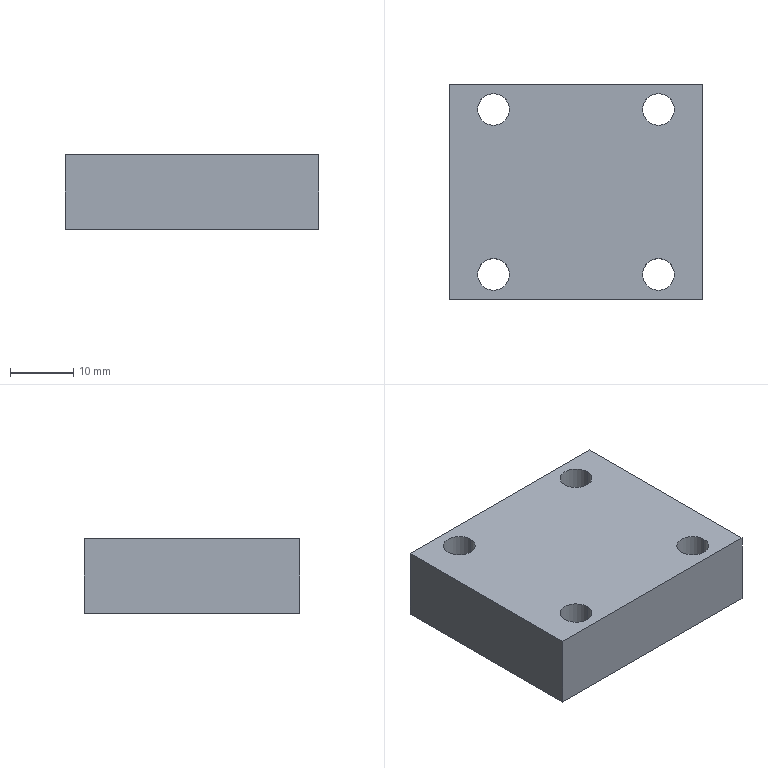Part | NX | 1 solid | 14 faces | box 40 x 34 x 11.7 mm | volume 14993 mm3 | cylinder 8 | plane 6 | commonest cylinder face diameters 5 x8
STEP:
#1=CARTESIAN_POINT('',(0.,-34.,12.3));
#2=VERTEX_POINT('',#1);
#3=CARTESIAN_POINT('',(0.,0.,12.3));
#4=VERTEX_POINT('',#3);
#5=CARTESIAN_POINT('',(0.,0.,12.3));
#6=DIRECTION('',(0.,1.,0.));
#7=VECTOR('',#6,1000.);
#8=LINE('',#5,#7);
#9=EDGE_CURVE('',#2,#4,#8,.T.);
#10=ORIENTED_EDGE('',*,*,#9,.F.);
#11=CARTESIAN_POINT('',(40.,-34.,12.3));
#12=VERTEX_POINT('',#11);
#13=CARTESIAN_POINT('',(0.,-34.,12.3));
#14=DIRECTION('',(1.,0.,0.));
#15=VECTOR('',#14,1000.);
#16=LINE('',#13,#15);
#17=EDGE_CURVE('',#2,#12,#16,.T.);
#18=ORIENTED_EDGE('',*,*,#17,.T.);
#19=CARTESIAN_POINT('',(40.,0.,12.3));
#20=VERTEX_POINT('',#19);
#21=CARTESIAN_POINT('',(40.,0.,12.3));
#22=DIRECTION('',(0.,-1.,0.));
#23=VECTOR('',#22,1000.);
#24=LINE('',#21,#23);
#25=EDGE_CURVE('',#20,#12,#24,.T.);
#26=ORIENTED_EDGE('',*,*,#25,.F.);
#27=CARTESIAN_POINT('',(0.,0.,12.3));
#28=DIRECTION('',(1.,0.,0.));
#29=VECTOR('',#28,1000.);
#30=LINE('',#27,#29);
#31=EDGE_CURVE('',#4,#20,#30,.T.);
#32=ORIENTED_EDGE('',*,*,#31,.F.);
#33=EDGE_LOOP('',(#10,#18,#26,#32));
#34=FACE_BOUND('',#33,.T.);
#35=CARTESIAN_POINT('',(4.5,-4.,12.3));
#36=VERTEX_POINT('',#35);
#37=CARTESIAN_POINT('',(9.5,-4.,12.3));
#38=VERTEX_POINT('',#37);
#39=CARTESIAN_POINT('',(7.,-4.,12.3));
#40=DIRECTION('',(0.,0.,-1.));
#41=DIRECTION('',(-1.,0.,0.));
#42=AXIS2_PLACEMENT_3D('',#39,#40,#41);
#43=CIRCLE('',#42,2.5);
#44=EDGE_CURVE('',#36,#38,#43,.T.);
#45=ORIENTED_EDGE('',*,*,#44,.T.);
#46=CARTESIAN_POINT('',(7.,-4.,12.3));
#47=DIRECTION('',(0.,0.,-1.));
#48=DIRECTION('',(-1.,0.,0.));
#49=AXIS2_PLACEMENT_3D('',#46,#47,#48);
#50=CIRCLE('',#49,2.5);
#51=EDGE_CURVE('',#38,#36,#50,.T.);
#52=ORIENTED_EDGE('',*,*,#51,.T.);
#53=EDGE_LOOP('',(#45,#52));
#54=FACE_BOUND('',#53,.T.);
#55=CARTESIAN_POINT('',(35.5,-30.,12.3));
#56=VERTEX_POINT('',#55);
#57=CARTESIAN_POINT('',(30.5,-30.,12.3));
#58=VERTEX_POINT('',#57);
#59=CARTESIAN_POINT('',(33.,-30.,12.3));
#60=DIRECTION('',(0.,0.,-1.));
#61=DIRECTION('',(-1.,0.,0.));
#62=AXIS2_PLACEMENT_3D('',#59,#60,#61);
#63=CIRCLE('',#62,2.5);
#64=EDGE_CURVE('',#56,#58,#63,.T.);
#65=ORIENTED_EDGE('',*,*,#64,.T.);
#66=CARTESIAN_POINT('',(33.,-30.,12.3));
#67=DIRECTION('',(0.,0.,-1.));
#68=DIRECTION('',(-1.,0.,0.));
#69=AXIS2_PLACEMENT_3D('',#66,#67,#68);
#70=CIRCLE('',#69,2.5);
#71=EDGE_CURVE('',#58,#56,#70,.T.);
#72=ORIENTED_EDGE('',*,*,#71,.T.);
#73=EDGE_LOOP('',(#65,#72));
#74=FACE_BOUND('',#73,.T.);
#75=CARTESIAN_POINT('',(35.5,-4.,12.3));
#76=VERTEX_POINT('',#75);
#77=CARTESIAN_POINT('',(30.5,-4.,12.3));
#78=VERTEX_POINT('',#77);
#79=CARTESIAN_POINT('',(33.,-4.,12.3));
#80=DIRECTION('',(0.,0.,-1.));
#81=DIRECTION('',(-1.,0.,0.));
#82=AXIS2_PLACEMENT_3D('',#79,#80,#81);
#83=CIRCLE('',#82,2.5);
#84=EDGE_CURVE('',#76,#78,#83,.T.);
#85=ORIENTED_EDGE('',*,*,#84,.T.);
#86=CARTESIAN_POINT('',(33.,-4.,12.3));
#87=DIRECTION('',(0.,0.,-1.));
#88=DIRECTION('',(-1.,0.,0.));
#89=AXIS2_PLACEMENT_3D('',#86,#87,#88);
#90=CIRCLE('',#89,2.5);
#91=EDGE_CURVE('',#78,#76,#90,.T.);
#92=ORIENTED_EDGE('',*,*,#91,.T.);
#93=EDGE_LOOP('',(#85,#92));
#94=FACE_BOUND('',#93,.T.);
#95=CARTESIAN_POINT('',(9.5,-30.,12.3));
#96=VERTEX_POINT('',#95);
#97=CARTESIAN_POINT('',(4.5,-30.,12.3));
#98=VERTEX_POINT('',#97);
#99=CARTESIAN_POINT('',(7.,-30.,12.3));
#100=DIRECTION('',(0.,0.,-1.));
#101=DIRECTION('',(-1.,0.,0.));
#102=AXIS2_PLACEMENT_3D('',#99,#100,#101);
#103=CIRCLE('',#102,2.5);
#104=EDGE_CURVE('',#96,#98,#103,.T.);
#105=ORIENTED_EDGE('',*,*,#104,.T.);
#106=CARTESIAN_POINT('',(7.,-30.,12.3));
#107=DIRECTION('',(0.,0.,-1.));
#108=DIRECTION('',(-1.,0.,0.));
#109=AXIS2_PLACEMENT_3D('',#106,#107,#108);
#110=CIRCLE('',#109,2.5);
#111=EDGE_CURVE('',#98,#96,#110,.T.);
#112=ORIENTED_EDGE('',*,*,#111,.T.);
#113=EDGE_LOOP('',(#105,#112));
#114=FACE_BOUND('',#113,.T.);
#115=CARTESIAN_POINT('',(0.,0.,12.3));
#116=DIRECTION('',(0.,0.,1.));
#117=DIRECTION('',(1.,0.,0.));
#118=AXIS2_PLACEMENT_3D('',#115,#116,#117);
#119=PLANE('',#118);
#120=ADVANCED_FACE('',(#34,#54,#74,#94,#114),#119,.T.);
#121=CARTESIAN_POINT('',(0.,0.,0.6));
#122=VERTEX_POINT('',#121);
#123=CARTESIAN_POINT('',(0.,-34.,0.6));
#124=VERTEX_POINT('',#123);
#125=CARTESIAN_POINT('',(0.,0.,0.6));
#126=DIRECTION('',(0.,-1.,0.));
#127=VECTOR('',#126,1000.);
#128=LINE('',#125,#127);
#129=EDGE_CURVE('',#122,#124,#128,.T.);
#130=ORIENTED_EDGE('',*,*,#129,.T.);
#131=CARTESIAN_POINT('',(0.,-34.,0.));
#132=DIRECTION('',(0.,0.,1.));
#133=VECTOR('',#132,1000.);
#134=LINE('',#131,#133);
#135=EDGE_CURVE('',#124,#2,#134,.T.);
#136=ORIENTED_EDGE('',*,*,#135,.T.);
#137=ORIENTED_EDGE('',*,*,#9,.T.);
#138=CARTESIAN_POINT('',(0.,0.,0.));
#139=DIRECTION('',(0.,0.,1.));
#140=VECTOR('',#139,1000.);
#141=LINE('',#138,#140);
#142=EDGE_CURVE('',#122,#4,#141,.T.);
#143=ORIENTED_EDGE('',*,*,#142,.F.);
#144=EDGE_LOOP('',(#130,#136,#137,#143));
#145=FACE_BOUND('',#144,.T.);
#146=CARTESIAN_POINT('',(0.,0.,0.));
#147=DIRECTION('',(-1.,0.,0.));
#148=DIRECTION('',(0.,0.,1.));
#149=AXIS2_PLACEMENT_3D('',#146,#147,#148);
#150=PLANE('',#149);
#151=ADVANCED_FACE('',(#145),#150,.T.);
#152=CARTESIAN_POINT('',(40.,0.,0.6));
#153=VERTEX_POINT('',#152);
#154=CARTESIAN_POINT('',(0.,0.,0.6));
#155=DIRECTION('',(-1.,0.,0.));
#156=VECTOR('',#155,1000.);
#157=LINE('',#154,#156);
#158=EDGE_CURVE('',#153,#122,#157,.T.);
#159=ORIENTED_EDGE('',*,*,#158,.T.);
#160=ORIENTED_EDGE('',*,*,#142,.T.);
#161=ORIENTED_EDGE('',*,*,#31,.T.);
#162=CARTESIAN_POINT('',(40.,0.,0.));
#163=DIRECTION('',(0.,0.,-1.));
#164=VECTOR('',#163,1000.);
#165=LINE('',#162,#164);
#166=EDGE_CURVE('',#20,#153,#165,.T.);
#167=ORIENTED_EDGE('',*,*,#166,.T.);
#168=EDGE_LOOP('',(#159,#160,#161,#167));
#169=FACE_BOUND('',#168,.T.);
#170=CARTESIAN_POINT('',(40.,0.,0.));
#171=DIRECTION('',(0.,1.,0.));
#172=DIRECTION('',(1.,0.,0.));
#173=AXIS2_PLACEMENT_3D('',#170,#171,#172);
#174=PLANE('',#173);
#175=ADVANCED_FACE('',(#169),#174,.T.);
#176=CARTESIAN_POINT('',(40.,-34.,0.6));
#177=VERTEX_POINT('',#176);
#178=CARTESIAN_POINT('',(40.,0.,0.6));
#179=DIRECTION('',(0.,1.,0.));
#180=VECTOR('',#179,1000.);
#181=LINE('',#178,#180);
#182=EDGE_CURVE('',#177,#153,#181,.T.);
#183=ORIENTED_EDGE('',*,*,#182,.T.);
#184=ORIENTED_EDGE('',*,*,#166,.F.);
#185=ORIENTED_EDGE('',*,*,#25,.T.);
#186=CARTESIAN_POINT('',(40.,-34.,0.));
#187=DIRECTION('',(0.,0.,-1.));
#188=VECTOR('',#187,1000.);
#189=LINE('',#186,#188);
#190=EDGE_CURVE('',#12,#177,#189,.T.);
#191=ORIENTED_EDGE('',*,*,#190,.T.);
#192=EDGE_LOOP('',(#183,#184,#185,#191));
#193=FACE_BOUND('',#192,.T.);
#194=CARTESIAN_POINT('',(40.,-34.,0.));
#195=DIRECTION('',(1.,0.,0.));
#196=DIRECTION('',(0.,1.,0.));
#197=AXIS2_PLACEMENT_3D('',#194,#195,#196);
#198=PLANE('',#197);
#199=ADVANCED_FACE('',(#193),#198,.T.);
#200=CARTESIAN_POINT('',(0.,-34.,0.6));
#201=DIRECTION('',(1.,0.,0.));
#202=VECTOR('',#201,1000.);
#203=LINE('',#200,#202);
#204=EDGE_CURVE('',#124,#177,#203,.T.);
#205=ORIENTED_EDGE('',*,*,#204,.T.);
#206=ORIENTED_EDGE('',*,*,#190,.F.);
#207=ORIENTED_EDGE('',*,*,#17,.F.);
#208=ORIENTED_EDGE('',*,*,#135,.F.);
#209=EDGE_LOOP('',(#205,#206,#207,#208));
#210=FACE_BOUND('',#209,.T.);
#211=CARTESIAN_POINT('',(0.,-34.,0.));
#212=DIRECTION('',(0.,-1.,0.));
#213=DIRECTION('',(0.,0.,-1.));
#214=AXIS2_PLACEMENT_3D('',#211,#212,#213);
#215=PLANE('',#214);
#216=ADVANCED_FACE('',(#210),#215,.T.);
#217=ORIENTED_EDGE('',*,*,#129,.F.);
#218=ORIENTED_EDGE('',*,*,#158,.F.);
#219=ORIENTED_EDGE('',*,*,#182,.F.);
#220=ORIENTED_EDGE('',*,*,#204,.F.);
#221=EDGE_LOOP('',(#217,#218,#219,#220));
#222=FACE_BOUND('',#221,.T.);
#223=CARTESIAN_POINT('',(9.5,-4.,0.6));
#224=VERTEX_POINT('',#223);
#225=CARTESIAN_POINT('',(4.5,-4.,0.6));
#226=VERTEX_POINT('',#225);
#227=CARTESIAN_POINT('',(7.,-4.,0.6));
#228=DIRECTION('',(0.,0.,-1.));
#229=DIRECTION('',(-1.,0.,0.));
#230=AXIS2_PLACEMENT_3D('',#227,#228,#229);
#231=CIRCLE('',#230,2.5);
#232=EDGE_CURVE('',#224,#226,#231,.T.);
#233=ORIENTED_EDGE('',*,*,#232,.F.);
#234=CARTESIAN_POINT('',(7.,-4.,0.6));
#235=DIRECTION('',(0.,0.,-1.));
#236=DIRECTION('',(-1.,0.,0.));
#237=AXIS2_PLACEMENT_3D('',#234,#235,#236);
#238=CIRCLE('',#237,2.5);
#239=EDGE_CURVE('',#226,#224,#238,.T.);
#240=ORIENTED_EDGE('',*,*,#239,.F.);
#241=EDGE_LOOP('',(#233,#240));
#242=FACE_BOUND('',#241,.T.);
#243=CARTESIAN_POINT('',(30.5,-30.,0.6));
#244=VERTEX_POINT('',#243);
#245=CARTESIAN_POINT('',(35.5,-30.,0.6));
#246=VERTEX_POINT('',#245);
#247=CARTESIAN_POINT('',(33.,-30.,0.6));
#248=DIRECTION('',(0.,0.,-1.));
#249=DIRECTION('',(-1.,0.,0.));
#250=AXIS2_PLACEMENT_3D('',#247,#248,#249);
#251=CIRCLE('',#250,2.5);
#252=EDGE_CURVE('',#244,#246,#251,.T.);
#253=ORIENTED_EDGE('',*,*,#252,.F.);
#254=CARTESIAN_POINT('',(33.,-30.,0.6));
#255=DIRECTION('',(0.,0.,-1.));
#256=DIRECTION('',(-1.,0.,0.));
#257=AXIS2_PLACEMENT_3D('',#254,#255,#256);
#258=CIRCLE('',#257,2.5);
#259=EDGE_CURVE('',#246,#244,#258,.T.);
#260=ORIENTED_EDGE('',*,*,#259,.F.);
#261=EDGE_LOOP('',(#253,#260));
#262=FACE_BOUND('',#261,.T.);
#263=CARTESIAN_POINT('',(35.5,-4.,0.6));
#264=VERTEX_POINT('',#263);
#265=CARTESIAN_POINT('',(30.5,-4.,0.6));
#266=VERTEX_POINT('',#265);
#267=CARTESIAN_POINT('',(33.,-4.,0.6));
#268=DIRECTION('',(0.,0.,-1.));
#269=DIRECTION('',(-1.,0.,0.));
#270=AXIS2_PLACEMENT_3D('',#267,#268,#269);
#271=CIRCLE('',#270,2.5);
#272=EDGE_CURVE('',#264,#266,#271,.T.);
#273=ORIENTED_EDGE('',*,*,#272,.F.);
#274=CARTESIAN_POINT('',(33.,-4.,0.6));
#275=DIRECTION('',(0.,0.,-1.));
#276=DIRECTION('',(-1.,0.,0.));
#277=AXIS2_PLACEMENT_3D('',#274,#275,#276);
#278=CIRCLE('',#277,2.5);
#279=EDGE_CURVE('',#266,#264,#278,.T.);
#280=ORIENTED_EDGE('',*,*,#279,.F.);
#281=EDGE_LOOP('',(#273,#280));
#282=FACE_BOUND('',#281,.T.);
#283=CARTESIAN_POINT('',(9.5,-30.,0.6));
#284=VERTEX_POINT('',#283);
#285=CARTESIAN_POINT('',(4.5,-30.,0.6));
#286=VERTEX_POINT('',#285);
#287=CARTESIAN_POINT('',(7.,-30.,0.6));
#288=DIRECTION('',(0.,0.,-1.));
#289=DIRECTION('',(-1.,0.,0.));
#290=AXIS2_PLACEMENT_3D('',#287,#288,#289);
#291=CIRCLE('',#290,2.5);
#292=EDGE_CURVE('',#284,#286,#291,.T.);
#293=ORIENTED_EDGE('',*,*,#292,.F.);
#294=CARTESIAN_POINT('',(7.,-30.,0.6));
#295=DIRECTION('',(0.,0.,-1.));
#296=DIRECTION('',(-1.,0.,0.));
#297=AXIS2_PLACEMENT_3D('',#294,#295,#296);
#298=CIRCLE('',#297,2.5);
#299=EDGE_CURVE('',#286,#284,#298,.T.);
#300=ORIENTED_EDGE('',*,*,#299,.F.);
#301=EDGE_LOOP('',(#293,#300));
#302=FACE_BOUND('',#301,.T.);
#303=CARTESIAN_POINT('',(0.,0.,0.6));
#304=DIRECTION('',(0.,0.,1.));
#305=DIRECTION('',(1.,0.,0.));
#306=AXIS2_PLACEMENT_3D('',#303,#304,#305);
#307=PLANE('',#306);
#308=ADVANCED_FACE('',(#222,#242,#262,#282,#302),#307,.F.);
#309=ORIENTED_EDGE('',*,*,#232,.T.);
#310=CARTESIAN_POINT('',(4.5,-4.,3.7));
#311=DIRECTION('',(0.,0.,-1.));
#312=VECTOR('',#311,1000.);
#313=LINE('',#310,#312);
#314=EDGE_CURVE('',#226,#36,#313,.F.);
#315=ORIENTED_EDGE('',*,*,#314,.T.);
#316=ORIENTED_EDGE('',*,*,#51,.F.);
#317=CARTESIAN_POINT('',(9.5,-4.,3.7));
#318=DIRECTION('',(0.,0.,-1.));
#319=VECTOR('',#318,1000.);
#320=LINE('',#317,#319);
#321=EDGE_CURVE('',#224,#38,#320,.F.);
#322=ORIENTED_EDGE('',*,*,#321,.F.);
#323=EDGE_LOOP('',(#309,#315,#316,#322));
#324=FACE_BOUND('',#323,.T.);
#325=CARTESIAN_POINT('',(7.,-4.,3.7));
#326=DIRECTION('',(0.,0.,-1.));
#327=DIRECTION('',(-1.,0.,0.));
#328=AXIS2_PLACEMENT_3D('',#325,#326,#327);
#329=CYLINDRICAL_SURFACE('',#328,2.5);
#330=ADVANCED_FACE('',(#324),#329,.F.);
#331=ORIENTED_EDGE('',*,*,#84,.F.);
#332=CARTESIAN_POINT('',(35.5,-4.,3.7));
#333=DIRECTION('',(0.,0.,-1.));
#334=VECTOR('',#333,1000.);
#335=LINE('',#332,#334);
#336=EDGE_CURVE('',#264,#76,#335,.F.);
#337=ORIENTED_EDGE('',*,*,#336,.F.);
#338=ORIENTED_EDGE('',*,*,#272,.T.);
#339=CARTESIAN_POINT('',(30.5,-4.,3.7));
#340=DIRECTION('',(0.,0.,-1.));
#341=VECTOR('',#340,1000.);
#342=LINE('',#339,#341);
#343=EDGE_CURVE('',#266,#78,#342,.F.);
#344=ORIENTED_EDGE('',*,*,#343,.T.);
#345=EDGE_LOOP('',(#331,#337,#338,#344));
#346=FACE_BOUND('',#345,.T.);
#347=CARTESIAN_POINT('',(33.,-4.,3.7));
#348=DIRECTION('',(0.,0.,-1.));
#349=DIRECTION('',(-1.,0.,0.));
#350=AXIS2_PLACEMENT_3D('',#347,#348,#349);
#351=CYLINDRICAL_SURFACE('',#350,2.5);
#352=ADVANCED_FACE('',(#346),#351,.F.);
#353=ORIENTED_EDGE('',*,*,#292,.T.);
#354=CARTESIAN_POINT('',(4.5,-30.,3.7));
#355=DIRECTION('',(0.,0.,-1.));
#356=VECTOR('',#355,1000.);
#357=LINE('',#354,#356);
#358=EDGE_CURVE('',#286,#98,#357,.F.);
#359=ORIENTED_EDGE('',*,*,#358,.T.);
#360=ORIENTED_EDGE('',*,*,#104,.F.);
#361=CARTESIAN_POINT('',(9.5,-30.,3.7));
#362=DIRECTION('',(0.,0.,-1.));
#363=VECTOR('',#362,1000.);
#364=LINE('',#361,#363);
#365=EDGE_CURVE('',#284,#96,#364,.F.);
#366=ORIENTED_EDGE('',*,*,#365,.F.);
#367=EDGE_LOOP('',(#353,#359,#360,#366));
#368=FACE_BOUND('',#367,.T.);
#369=CARTESIAN_POINT('',(7.,-30.,3.7));
#370=DIRECTION('',(0.,0.,-1.));
#371=DIRECTION('',(-1.,0.,0.));
#372=AXIS2_PLACEMENT_3D('',#369,#370,#371);
#373=CYLINDRICAL_SURFACE('',#372,2.5);
#374=ADVANCED_FACE('',(#368),#373,.F.);
#375=ORIENTED_EDGE('',*,*,#64,.F.);
#376=CARTESIAN_POINT('',(35.5,-30.,3.7));
#377=DIRECTION('',(0.,0.,-1.));
#378=VECTOR('',#377,1000.);
#379=LINE('',#376,#378);
#380=EDGE_CURVE('',#56,#246,#379,.T.);
#381=ORIENTED_EDGE('',*,*,#380,.T.);
#382=ORIENTED_EDGE('',*,*,#259,.T.);
#383=CARTESIAN_POINT('',(30.5,-30.,3.7));
#384=DIRECTION('',(0.,0.,-1.));
#385=VECTOR('',#384,1000.);
#386=LINE('',#383,#385);
#387=EDGE_CURVE('',#58,#244,#386,.T.);
#388=ORIENTED_EDGE('',*,*,#387,.F.);
#389=EDGE_LOOP('',(#375,#381,#382,#388));
#390=FACE_BOUND('',#389,.T.);
#391=CARTESIAN_POINT('',(33.,-30.,3.7));
#392=DIRECTION('',(0.,0.,-1.));
#393=DIRECTION('',(-1.,0.,0.));
#394=AXIS2_PLACEMENT_3D('',#391,#392,#393);
#395=CYLINDRICAL_SURFACE('',#394,2.5);
#396=ADVANCED_FACE('',(#390),#395,.F.);
#397=ORIENTED_EDGE('',*,*,#343,.F.);
#398=ORIENTED_EDGE('',*,*,#279,.T.);
#399=ORIENTED_EDGE('',*,*,#336,.T.);
#400=ORIENTED_EDGE('',*,*,#91,.F.);
#401=EDGE_LOOP('',(#397,#398,#399,#400));
#402=FACE_BOUND('',#401,.T.);
#403=CARTESIAN_POINT('',(33.,-4.,3.7));
#404=DIRECTION('',(0.,0.,-1.));
#405=DIRECTION('',(-1.,0.,0.));
#406=AXIS2_PLACEMENT_3D('',#403,#404,#405);
#407=CYLINDRICAL_SURFACE('',#406,2.5);
#408=ADVANCED_FACE('',(#402),#407,.F.);
#409=ORIENTED_EDGE('',*,*,#252,.T.);
#410=ORIENTED_EDGE('',*,*,#380,.F.);
#411=ORIENTED_EDGE('',*,*,#71,.F.);
#412=ORIENTED_EDGE('',*,*,#387,.T.);
#413=EDGE_LOOP('',(#409,#410,#411,#412));
#414=FACE_BOUND('',#413,.T.);
#415=CARTESIAN_POINT('',(33.,-30.,3.7));
#416=DIRECTION('',(0.,0.,-1.));
#417=DIRECTION('',(-1.,0.,0.));
#418=AXIS2_PLACEMENT_3D('',#415,#416,#417);
#419=CYLINDRICAL_SURFACE('',#418,2.5);
#420=ADVANCED_FACE('',(#414),#419,.F.);
#421=ORIENTED_EDGE('',*,*,#44,.F.);
#422=ORIENTED_EDGE('',*,*,#314,.F.);
#423=ORIENTED_EDGE('',*,*,#239,.T.);
#424=ORIENTED_EDGE('',*,*,#321,.T.);
#425=EDGE_LOOP('',(#421,#422,#423,#424));
#426=FACE_BOUND('',#425,.T.);
#427=CARTESIAN_POINT('',(7.,-4.,3.7));
#428=DIRECTION('',(0.,0.,-1.));
#429=DIRECTION('',(-1.,0.,0.));
#430=AXIS2_PLACEMENT_3D('',#427,#428,#429);
#431=CYLINDRICAL_SURFACE('',#430,2.5);
#432=ADVANCED_FACE('',(#426),#431,.F.);
#433=ORIENTED_EDGE('',*,*,#358,.F.);
#434=ORIENTED_EDGE('',*,*,#299,.T.);
#435=ORIENTED_EDGE('',*,*,#365,.T.);
#436=ORIENTED_EDGE('',*,*,#111,.F.);
#437=EDGE_LOOP('',(#433,#434,#435,#436));
#438=FACE_BOUND('',#437,.T.);
#439=CARTESIAN_POINT('',(7.,-30.,3.7));
#440=DIRECTION('',(0.,0.,-1.));
#441=DIRECTION('',(-1.,0.,0.));
#442=AXIS2_PLACEMENT_3D('',#439,#440,#441);
#443=CYLINDRICAL_SURFACE('',#442,2.5);
#444=ADVANCED_FACE('',(#438),#443,.F.);
#445=CLOSED_SHELL('',(#120,#151,#175,#199,#216,#308,#330,#352,#374,#396,#408,#420,#432,#444));
#446=MANIFOLD_SOLID_BREP('',#445);
#447=(LENGTH_UNIT()NAMED_UNIT(*)SI_UNIT(.MILLI.,.METRE.));
#448=UNCERTAINTY_MEASURE_WITH_UNIT(LENGTH_MEASURE(0.00001),#447,'','');
#449=(NAMED_UNIT(*)PLANE_ANGLE_UNIT()SI_UNIT($,.RADIAN.));
#450=(NAMED_UNIT(*)SI_UNIT($,.STERADIAN.)SOLID_ANGLE_UNIT());
#451=(GEOMETRIC_REPRESENTATION_CONTEXT(3)GLOBAL_UNCERTAINTY_ASSIGNED_CONTEXT((#448))GLOBAL_UNIT_ASSIGNED_CONTEXT((#447,#449,#450))REPRESENTATION_CONTEXT('',''));
#452=ADVANCED_BREP_SHAPE_REPRESENTATION('',(#446),#451);